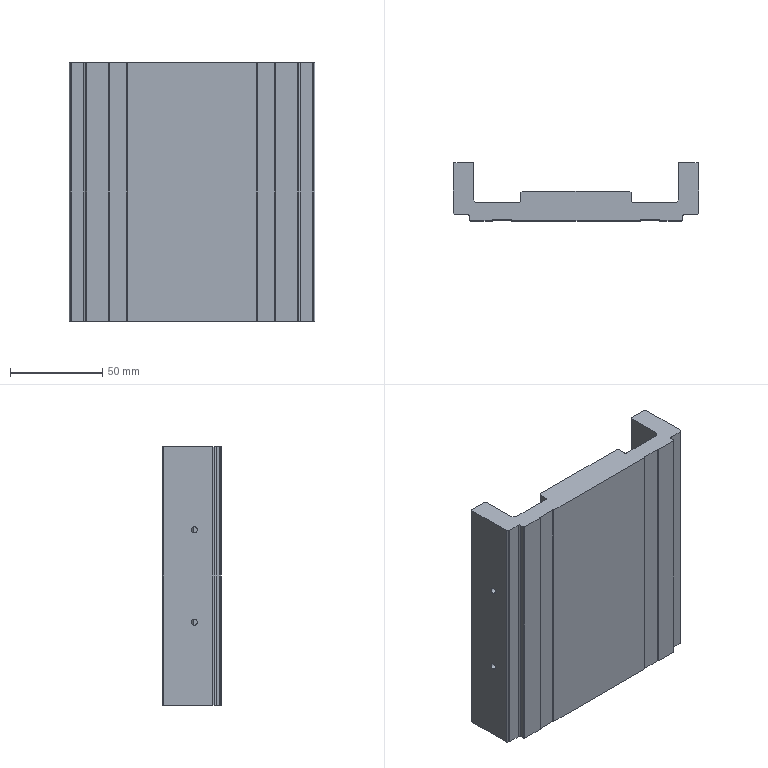Part | STEP file | 1 solid | 108 faces | box 133 x 31.5 x 140 mm | volume 288957 mm3 | cylinder 54 | plane 34 | cone 20 | commonest cylinder face diameters 0.6 x18 5 x16 3.3 x8 1 x4 2 x4 6 x4